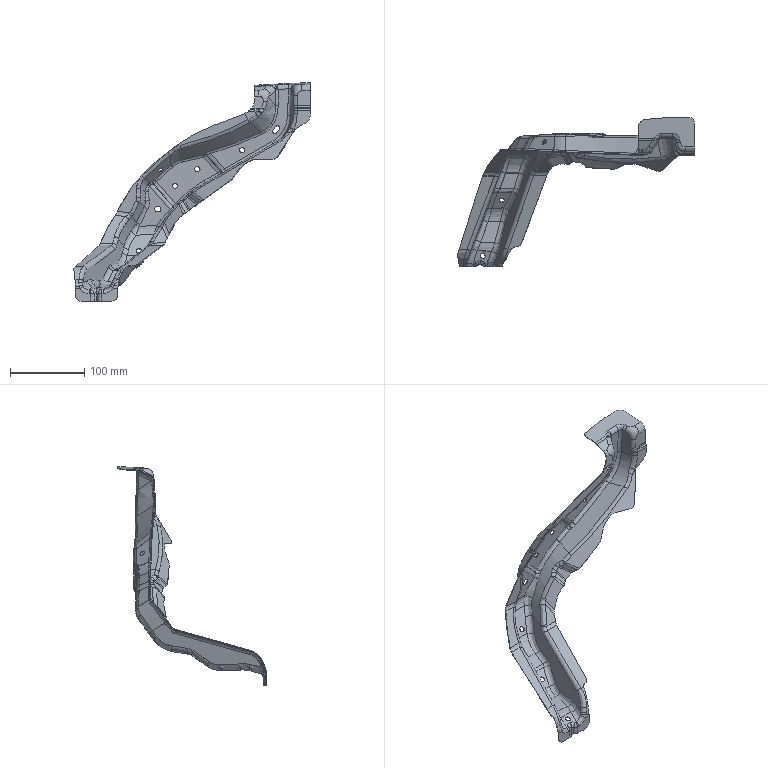Part | 1 solid | 510 faces | box 318.982 x 201.087 x 294.399 mm | volume 47142 mm3 | spline 290 | cylinder 138 | plane 67 | sphere 12 | other 3 | commonest cylinder face diameters 10 x29 11.6 x20 7 x14 16 x11 20 x10 8.4 x9